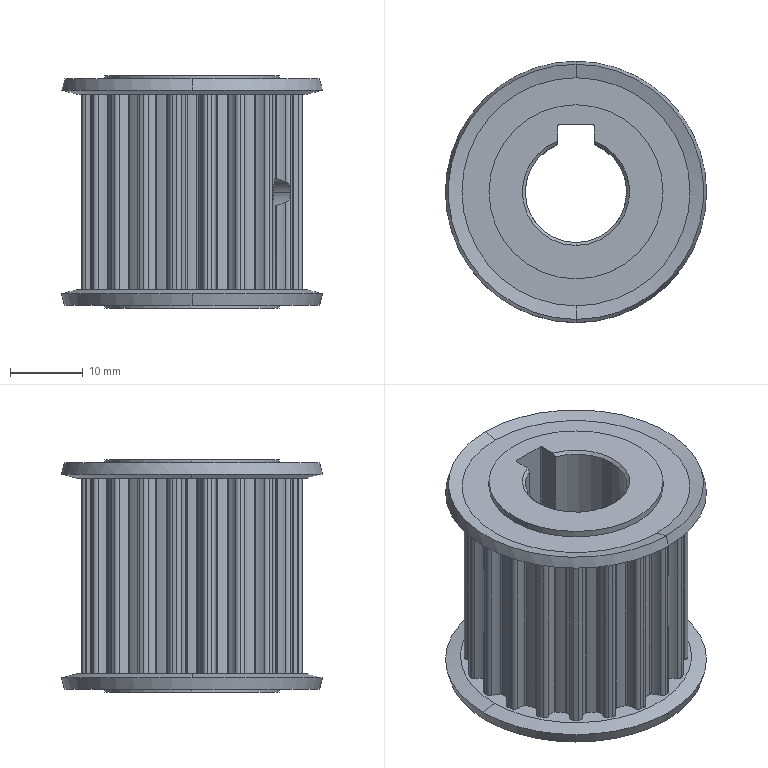Part | SolidWorks | features BaseBody 1 | 1 solid | 231 faces | box 36 x 36 x 32 mm | volume 16182 mm3 | cylinder 205 | cone 17 | plane 9 | commonest cylinder face diameters 1.1 x51 0.5 x50 6.55 x48 27.33 x23 30.87 x20 4.134 x4